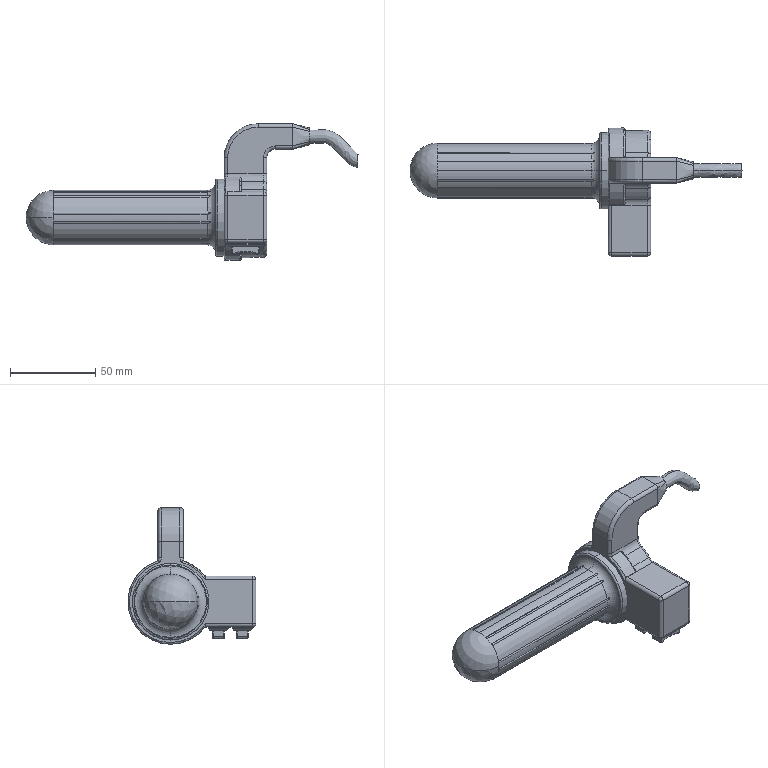Part | NX | features BREP 1 | 1 solid | 229 faces | box 194.399 x 75 x 80 mm | volume 130735 mm3 | cylinder 90 | plane 67 | torus 33 | spline 29 | sphere 6 | cone 4 | commonest cylinder face diameters 1.414 x16 4 x16 32 x13 0.4 x11 1 x8 10 x5